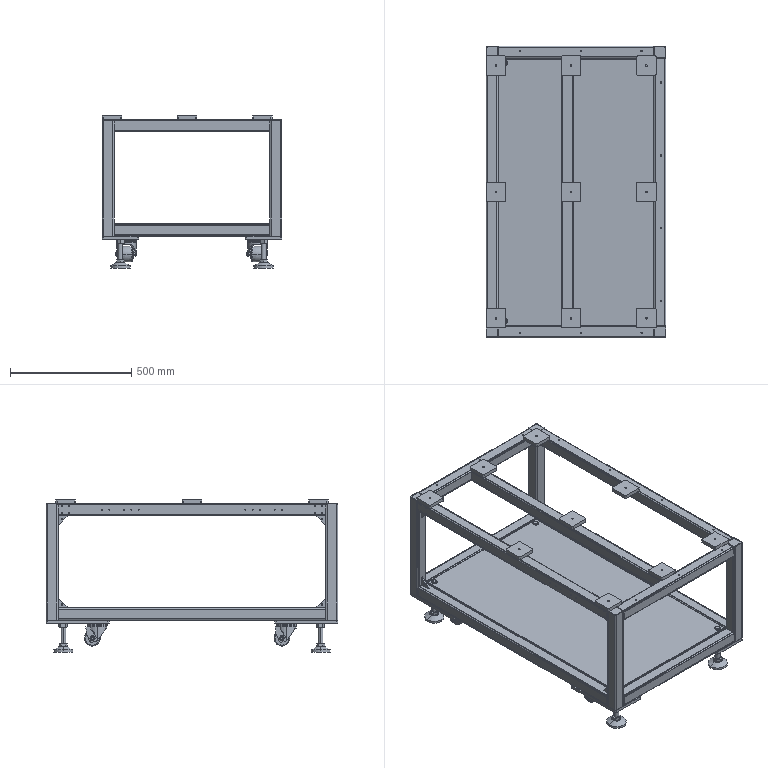Part | SolidWorks | features InContextFeatHolder 2 | 62 solids | 1773 faces | box 740 x 1200 x 627 mm | volume 11363553 mm3 | plane 687 | cylinder 602 | spline 356 | cone 112 | torus 16 | commonest cylinder face diameters 12 x92 6 x68 11 x48 5 x44 10 x36 8.5 x32